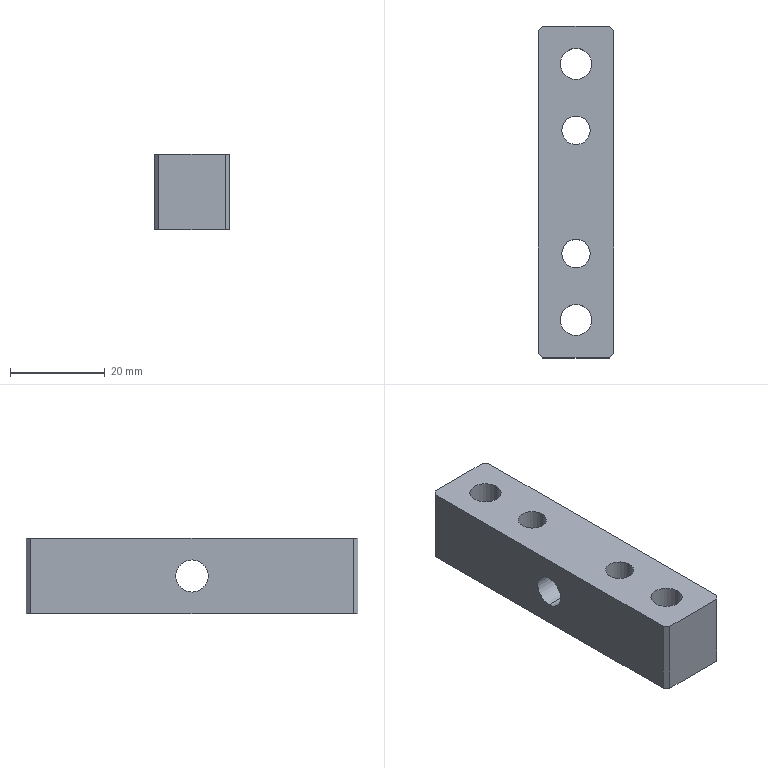Part | SolidWorks | features HoleWzd 3, Chamfer 1, ExtruThin 1 | 1 solid | 20 faces | box 16 x 70 x 16 mm | volume 15307 mm3 | cylinder 10 | plane 10 | commonest cylinder face diameters 6 x4 6.6 x4 6.8 x2
STEP:
#1=CARTESIAN_POINT('',(-11.3,62.,0.));
#2=VERTEX_POINT('',#1);
#3=CARTESIAN_POINT('',(-4.7,62.,0.));
#4=VERTEX_POINT('',#3);
#5=CARTESIAN_POINT('',(-8.,62.,0.));
#6=DIRECTION('',(0.,0.,1.));
#7=DIRECTION('',(1.,0.,0.));
#8=AXIS2_PLACEMENT_3D('',#5,#6,#7);
#9=CIRCLE('',#8,3.3);
#10=EDGE_CURVE('',#2,#4,#9,.T.);
#11=ORIENTED_EDGE('',*,*,#10,.F.);
#12=CARTESIAN_POINT('',(-11.3,62.,16.));
#13=VERTEX_POINT('',#12);
#14=CARTESIAN_POINT('',(-11.3,62.,16.));
#15=DIRECTION('',(0.,0.,1.));
#16=VECTOR('',#15,1000.);
#17=LINE('',#14,#16);
#18=EDGE_CURVE('',#2,#13,#17,.T.);
#19=ORIENTED_EDGE('',*,*,#18,.T.);
#20=CARTESIAN_POINT('',(-4.7,62.,16.));
#21=VERTEX_POINT('',#20);
#22=CARTESIAN_POINT('',(-8.,62.,16.));
#23=DIRECTION('',(0.,0.,1.));
#24=DIRECTION('',(1.,0.,0.));
#25=AXIS2_PLACEMENT_3D('',#22,#23,#24);
#26=CIRCLE('',#25,3.3);
#27=EDGE_CURVE('',#13,#21,#26,.T.);
#28=ORIENTED_EDGE('',*,*,#27,.T.);
#29=CARTESIAN_POINT('',(-4.7,62.,16.));
#30=DIRECTION('',(0.,0.,1.));
#31=VECTOR('',#30,1000.);
#32=LINE('',#29,#31);
#33=EDGE_CURVE('',#4,#21,#32,.T.);
#34=ORIENTED_EDGE('',*,*,#33,.F.);
#35=EDGE_LOOP('',(#11,#19,#28,#34));
#36=FACE_OUTER_BOUND('',#35,.T.);
#37=CARTESIAN_POINT('',(-8.,62.,16.));
#38=DIRECTION('',(0.,0.,1.));
#39=DIRECTION('',(1.,0.,0.));
#40=AXIS2_PLACEMENT_3D('',#37,#38,#39);
#41=CYLINDRICAL_SURFACE('',#40,3.3);
#42=ADVANCED_FACE('',(#36),#41,.F.);
#43=CARTESIAN_POINT('',(-11.3,8.,0.));
#44=VERTEX_POINT('',#43);
#45=CARTESIAN_POINT('',(-4.7,8.,0.));
#46=VERTEX_POINT('',#45);
#47=CARTESIAN_POINT('',(-8.,8.,0.));
#48=DIRECTION('',(0.,0.,1.));
#49=DIRECTION('',(1.,0.,0.));
#50=AXIS2_PLACEMENT_3D('',#47,#48,#49);
#51=CIRCLE('',#50,3.3);
#52=EDGE_CURVE('',#44,#46,#51,.T.);
#53=ORIENTED_EDGE('',*,*,#52,.F.);
#54=CARTESIAN_POINT('',(-11.3,8.,16.));
#55=VERTEX_POINT('',#54);
#56=CARTESIAN_POINT('',(-11.3,8.,16.));
#57=DIRECTION('',(0.,0.,1.));
#58=VECTOR('',#57,1000.);
#59=LINE('',#56,#58);
#60=EDGE_CURVE('',#44,#55,#59,.T.);
#61=ORIENTED_EDGE('',*,*,#60,.T.);
#62=CARTESIAN_POINT('',(-4.7,8.,16.));
#63=VERTEX_POINT('',#62);
#64=CARTESIAN_POINT('',(-8.,8.,16.));
#65=DIRECTION('',(0.,0.,1.));
#66=DIRECTION('',(1.,0.,0.));
#67=AXIS2_PLACEMENT_3D('',#64,#65,#66);
#68=CIRCLE('',#67,3.3);
#69=EDGE_CURVE('',#55,#63,#68,.T.);
#70=ORIENTED_EDGE('',*,*,#69,.T.);
#71=CARTESIAN_POINT('',(-4.7,8.,16.));
#72=DIRECTION('',(0.,0.,1.));
#73=VECTOR('',#72,1000.);
#74=LINE('',#71,#73);
#75=EDGE_CURVE('',#46,#63,#74,.T.);
#76=ORIENTED_EDGE('',*,*,#75,.F.);
#77=EDGE_LOOP('',(#53,#61,#70,#76));
#78=FACE_OUTER_BOUND('',#77,.T.);
#79=CARTESIAN_POINT('',(-8.,8.,16.));
#80=DIRECTION('',(0.,0.,1.));
#81=DIRECTION('',(1.,0.,0.));
#82=AXIS2_PLACEMENT_3D('',#79,#80,#81);
#83=CYLINDRICAL_SURFACE('',#82,3.3);
#84=ADVANCED_FACE('',(#78),#83,.F.);
#85=CARTESIAN_POINT('',(0.,35.,4.6));
#86=VERTEX_POINT('',#85);
#87=CARTESIAN_POINT('',(0.,35.,11.4));
#88=VERTEX_POINT('',#87);
#89=CARTESIAN_POINT('',(0.,35.,8.));
#90=DIRECTION('',(-1.,0.,0.));
#91=DIRECTION('',(0.,0.,1.));
#92=AXIS2_PLACEMENT_3D('',#89,#90,#91);
#93=CIRCLE('',#92,3.4);
#94=EDGE_CURVE('',#86,#88,#93,.T.);
#95=ORIENTED_EDGE('',*,*,#94,.F.);
#96=CARTESIAN_POINT('',(-16.,35.,4.6));
#97=VERTEX_POINT('',#96);
#98=CARTESIAN_POINT('',(-16.,35.,4.6));
#99=DIRECTION('',(-1.,0.,0.));
#100=VECTOR('',#99,1000.);
#101=LINE('',#98,#100);
#102=EDGE_CURVE('',#86,#97,#101,.T.);
#103=ORIENTED_EDGE('',*,*,#102,.T.);
#104=CARTESIAN_POINT('',(-16.,35.,11.4));
#105=VERTEX_POINT('',#104);
#106=CARTESIAN_POINT('',(-16.,35.,8.));
#107=DIRECTION('',(-1.,0.,0.));
#108=DIRECTION('',(0.,0.,1.));
#109=AXIS2_PLACEMENT_3D('',#106,#107,#108);
#110=CIRCLE('',#109,3.4);
#111=EDGE_CURVE('',#97,#105,#110,.T.);
#112=ORIENTED_EDGE('',*,*,#111,.T.);
#113=CARTESIAN_POINT('',(-16.,35.,11.4));
#114=DIRECTION('',(-1.,0.,0.));
#115=VECTOR('',#114,1000.);
#116=LINE('',#113,#115);
#117=EDGE_CURVE('',#88,#105,#116,.T.);
#118=ORIENTED_EDGE('',*,*,#117,.F.);
#119=EDGE_LOOP('',(#95,#103,#112,#118));
#120=FACE_OUTER_BOUND('',#119,.T.);
#121=CARTESIAN_POINT('',(-16.,35.,8.));
#122=DIRECTION('',(-1.,0.,0.));
#123=DIRECTION('',(0.,0.,1.));
#124=AXIS2_PLACEMENT_3D('',#121,#122,#123);
#125=CYLINDRICAL_SURFACE('',#124,3.4);
#126=ADVANCED_FACE('',(#120),#125,.F.);
#127=CARTESIAN_POINT('',(-11.,48.,0.));
#128=VERTEX_POINT('',#127);
#129=CARTESIAN_POINT('',(-5.,48.,0.));
#130=VERTEX_POINT('',#129);
#131=CARTESIAN_POINT('',(-8.,48.,0.));
#132=DIRECTION('',(0.,0.,1.));
#133=DIRECTION('',(1.,0.,0.));
#134=AXIS2_PLACEMENT_3D('',#131,#132,#133);
#135=CIRCLE('',#134,3.);
#136=EDGE_CURVE('',#128,#130,#135,.T.);
#137=ORIENTED_EDGE('',*,*,#136,.F.);
#138=CARTESIAN_POINT('',(-11.,48.,16.));
#139=VERTEX_POINT('',#138);
#140=CARTESIAN_POINT('',(-11.,48.,16.));
#141=DIRECTION('',(0.,0.,1.));
#142=VECTOR('',#141,1000.);
#143=LINE('',#140,#142);
#144=EDGE_CURVE('',#128,#139,#143,.T.);
#145=ORIENTED_EDGE('',*,*,#144,.T.);
#146=CARTESIAN_POINT('',(-5.,48.,16.));
#147=VERTEX_POINT('',#146);
#148=CARTESIAN_POINT('',(-8.,48.,16.));
#149=DIRECTION('',(0.,0.,1.));
#150=DIRECTION('',(1.,0.,0.));
#151=AXIS2_PLACEMENT_3D('',#148,#149,#150);
#152=CIRCLE('',#151,3.);
#153=EDGE_CURVE('',#139,#147,#152,.T.);
#154=ORIENTED_EDGE('',*,*,#153,.T.);
#155=CARTESIAN_POINT('',(-5.,48.,16.));
#156=DIRECTION('',(0.,0.,1.));
#157=VECTOR('',#156,1000.);
#158=LINE('',#155,#157);
#159=EDGE_CURVE('',#130,#147,#158,.T.);
#160=ORIENTED_EDGE('',*,*,#159,.F.);
#161=EDGE_LOOP('',(#137,#145,#154,#160));
#162=FACE_OUTER_BOUND('',#161,.T.);
#163=CARTESIAN_POINT('',(-8.,48.,16.));
#164=DIRECTION('',(0.,0.,1.));
#165=DIRECTION('',(1.,0.,0.));
#166=AXIS2_PLACEMENT_3D('',#163,#164,#165);
#167=CYLINDRICAL_SURFACE('',#166,3.);
#168=ADVANCED_FACE('',(#162),#167,.F.);
#169=CARTESIAN_POINT('',(-11.,22.,0.));
#170=VERTEX_POINT('',#169);
#171=CARTESIAN_POINT('',(-5.,22.,0.));
#172=VERTEX_POINT('',#171);
#173=CARTESIAN_POINT('',(-8.,22.,0.));
#174=DIRECTION('',(0.,0.,1.));
#175=DIRECTION('',(1.,0.,0.));
#176=AXIS2_PLACEMENT_3D('',#173,#174,#175);
#177=CIRCLE('',#176,3.);
#178=EDGE_CURVE('',#170,#172,#177,.T.);
#179=ORIENTED_EDGE('',*,*,#178,.F.);
#180=CARTESIAN_POINT('',(-11.,22.,16.));
#181=VERTEX_POINT('',#180);
#182=CARTESIAN_POINT('',(-11.,22.,16.));
#183=DIRECTION('',(0.,0.,1.));
#184=VECTOR('',#183,1000.);
#185=LINE('',#182,#184);
#186=EDGE_CURVE('',#170,#181,#185,.T.);
#187=ORIENTED_EDGE('',*,*,#186,.T.);
#188=CARTESIAN_POINT('',(-5.,22.,16.));
#189=VERTEX_POINT('',#188);
#190=CARTESIAN_POINT('',(-8.,22.,16.));
#191=DIRECTION('',(0.,0.,1.));
#192=DIRECTION('',(1.,0.,0.));
#193=AXIS2_PLACEMENT_3D('',#190,#191,#192);
#194=CIRCLE('',#193,3.);
#195=EDGE_CURVE('',#181,#189,#194,.T.);
#196=ORIENTED_EDGE('',*,*,#195,.T.);
#197=CARTESIAN_POINT('',(-5.,22.,16.));
#198=DIRECTION('',(0.,0.,1.));
#199=VECTOR('',#198,1000.);
#200=LINE('',#197,#199);
#201=EDGE_CURVE('',#172,#189,#200,.T.);
#202=ORIENTED_EDGE('',*,*,#201,.F.);
#203=EDGE_LOOP('',(#179,#187,#196,#202));
#204=FACE_OUTER_BOUND('',#203,.T.);
#205=CARTESIAN_POINT('',(-8.,22.,16.));
#206=DIRECTION('',(0.,0.,1.));
#207=DIRECTION('',(1.,0.,0.));
#208=AXIS2_PLACEMENT_3D('',#205,#206,#207);
#209=CYLINDRICAL_SURFACE('',#208,3.);
#210=ADVANCED_FACE('',(#204),#209,.F.);
#211=CARTESIAN_POINT('',(-16.,35.,8.));
#212=DIRECTION('',(-1.,0.,0.));
#213=DIRECTION('',(0.,0.,1.));
#214=AXIS2_PLACEMENT_3D('',#211,#212,#213);
#215=CIRCLE('',#214,3.4);
#216=EDGE_CURVE('',#105,#97,#215,.T.);
#217=ORIENTED_EDGE('',*,*,#216,.F.);
#218=ORIENTED_EDGE('',*,*,#111,.F.);
#219=EDGE_LOOP('',(#217,#218));
#220=FACE_BOUND('',#219,.T.);
#221=CARTESIAN_POINT('',(-16.,69.,16.));
#222=VERTEX_POINT('',#221);
#223=CARTESIAN_POINT('',(-16.,1.,16.));
#224=VERTEX_POINT('',#223);
#225=CARTESIAN_POINT('',(-16.,70.,16.));
#226=DIRECTION('',(0.,-1.,0.));
#227=VECTOR('',#226,1000.);
#228=LINE('',#225,#227);
#229=EDGE_CURVE('',#222,#224,#228,.T.);
#230=ORIENTED_EDGE('',*,*,#229,.F.);
#231=CARTESIAN_POINT('',(-16.,69.,0.));
#232=VERTEX_POINT('',#231);
#233=CARTESIAN_POINT('',(-16.,69.,0.));
#234=DIRECTION('',(0.,0.,-1.));
#235=VECTOR('',#234,1000.);
#236=LINE('',#233,#235);
#237=EDGE_CURVE('',#222,#232,#236,.T.);
#238=ORIENTED_EDGE('',*,*,#237,.T.);
#239=CARTESIAN_POINT('',(-16.,1.,0.));
#240=VERTEX_POINT('',#239);
#241=CARTESIAN_POINT('',(-16.,70.,0.));
#242=DIRECTION('',(0.,-1.,0.));
#243=VECTOR('',#242,1000.);
#244=LINE('',#241,#243);
#245=EDGE_CURVE('',#232,#240,#244,.T.);
#246=ORIENTED_EDGE('',*,*,#245,.T.);
#247=CARTESIAN_POINT('',(-16.,1.,16.));
#248=DIRECTION('',(0.,0.,1.));
#249=VECTOR('',#248,1000.);
#250=LINE('',#247,#249);
#251=EDGE_CURVE('',#240,#224,#250,.T.);
#252=ORIENTED_EDGE('',*,*,#251,.T.);
#253=EDGE_LOOP('',(#230,#238,#246,#252));
#254=FACE_OUTER_BOUND('',#253,.T.);
#255=CARTESIAN_POINT('',(-16.,70.,16.));
#256=DIRECTION('',(1.,0.,0.));
#257=DIRECTION('',(0.,1.,0.));
#258=AXIS2_PLACEMENT_3D('',#255,#256,#257);
#259=PLANE('',#258);
#260=ADVANCED_FACE('',(#220,#254),#259,.F.);
#261=CARTESIAN_POINT('',(-1.,0.,0.));
#262=VERTEX_POINT('',#261);
#263=CARTESIAN_POINT('',(-15.,0.,0.));
#264=VERTEX_POINT('',#263);
#265=CARTESIAN_POINT('',(0.,0.,0.));
#266=DIRECTION('',(-1.,0.,0.));
#267=VECTOR('',#266,1000.);
#268=LINE('',#265,#267);
#269=EDGE_CURVE('',#262,#264,#268,.T.);
#270=ORIENTED_EDGE('',*,*,#269,.F.);
#271=CARTESIAN_POINT('',(-1.,0.,16.));
#272=VERTEX_POINT('',#271);
#273=CARTESIAN_POINT('',(-1.,0.,16.));
#274=DIRECTION('',(0.,0.,1.));
#275=VECTOR('',#274,1000.);
#276=LINE('',#273,#275);
#277=EDGE_CURVE('',#262,#272,#276,.T.);
#278=ORIENTED_EDGE('',*,*,#277,.T.);
#279=CARTESIAN_POINT('',(-15.,0.,16.));
#280=VERTEX_POINT('',#279);
#281=CARTESIAN_POINT('',(0.,0.,16.));
#282=DIRECTION('',(-1.,0.,0.));
#283=VECTOR('',#282,1000.);
#284=LINE('',#281,#283);
#285=EDGE_CURVE('',#272,#280,#284,.T.);
#286=ORIENTED_EDGE('',*,*,#285,.T.);
#287=CARTESIAN_POINT('',(-15.,0.,0.));
#288=DIRECTION('',(0.,0.,-1.));
#289=VECTOR('',#288,1000.);
#290=LINE('',#287,#289);
#291=EDGE_CURVE('',#280,#264,#290,.T.);
#292=ORIENTED_EDGE('',*,*,#291,.T.);
#293=EDGE_LOOP('',(#270,#278,#286,#292));
#294=FACE_OUTER_BOUND('',#293,.T.);
#295=CARTESIAN_POINT('',(0.,0.,16.));
#296=DIRECTION('',(0.,-1.,0.));
#297=DIRECTION('',(0.,0.,-1.));
#298=AXIS2_PLACEMENT_3D('',#295,#296,#297);
#299=PLANE('',#298);
#300=ADVANCED_FACE('',(#294),#299,.T.);
#301=CARTESIAN_POINT('',(0.,35.,8.));
#302=DIRECTION('',(-1.,0.,0.));
#303=DIRECTION('',(0.,0.,1.));
#304=AXIS2_PLACEMENT_3D('',#301,#302,#303);
#305=CIRCLE('',#304,3.4);
#306=EDGE_CURVE('',#88,#86,#305,.T.);
#307=ORIENTED_EDGE('',*,*,#306,.T.);
#308=ORIENTED_EDGE('',*,*,#94,.T.);
#309=EDGE_LOOP('',(#307,#308));
#310=FACE_BOUND('',#309,.T.);
#311=CARTESIAN_POINT('',(0.,69.,0.));
#312=VERTEX_POINT('',#311);
#313=CARTESIAN_POINT('',(0.,1.,0.));
#314=VERTEX_POINT('',#313);
#315=CARTESIAN_POINT('',(0.,70.,0.));
#316=DIRECTION('',(0.,-1.,0.));
#317=VECTOR('',#316,1000.);
#318=LINE('',#315,#317);
#319=EDGE_CURVE('',#312,#314,#318,.T.);
#320=ORIENTED_EDGE('',*,*,#319,.F.);
#321=CARTESIAN_POINT('',(0.,69.,16.));
#322=VERTEX_POINT('',#321);
#323=CARTESIAN_POINT('',(0.,69.,16.));
#324=DIRECTION('',(0.,0.,1.));
#325=VECTOR('',#324,1000.);
#326=LINE('',#323,#325);
#327=EDGE_CURVE('',#312,#322,#326,.T.);
#328=ORIENTED_EDGE('',*,*,#327,.T.);
#329=CARTESIAN_POINT('',(0.,1.,16.));
#330=VERTEX_POINT('',#329);
#331=CARTESIAN_POINT('',(0.,70.,16.));
#332=DIRECTION('',(0.,-1.,0.));
#333=VECTOR('',#332,1000.);
#334=LINE('',#331,#333);
#335=EDGE_CURVE('',#322,#330,#334,.T.);
#336=ORIENTED_EDGE('',*,*,#335,.T.);
#337=CARTESIAN_POINT('',(0.,1.,16.));
#338=DIRECTION('',(0.,0.,-1.));
#339=VECTOR('',#338,1000.);
#340=LINE('',#337,#339);
#341=EDGE_CURVE('',#330,#314,#340,.T.);
#342=ORIENTED_EDGE('',*,*,#341,.T.);
#343=EDGE_LOOP('',(#320,#328,#336,#342));
#344=FACE_OUTER_BOUND('',#343,.T.);
#345=CARTESIAN_POINT('',(0.,70.,16.));
#346=DIRECTION('',(1.,0.,0.));
#347=DIRECTION('',(0.,1.,0.));
#348=AXIS2_PLACEMENT_3D('',#345,#346,#347);
#349=PLANE('',#348);
#350=ADVANCED_FACE('',(#310,#344),#349,.T.);
#351=CARTESIAN_POINT('',(-15.,70.,0.));
#352=VERTEX_POINT('',#351);
#353=CARTESIAN_POINT('',(-1.,70.,0.));
#354=VERTEX_POINT('',#353);
#355=CARTESIAN_POINT('',(-16.,70.,0.));
#356=DIRECTION('',(1.,0.,0.));
#357=VECTOR('',#356,1000.);
#358=LINE('',#355,#357);
#359=EDGE_CURVE('',#352,#354,#358,.T.);
#360=ORIENTED_EDGE('',*,*,#359,.F.);
#361=CARTESIAN_POINT('',(-15.,70.,16.));
#362=VERTEX_POINT('',#361);
#363=CARTESIAN_POINT('',(-15.,70.,16.));
#364=DIRECTION('',(0.,0.,1.));
#365=VECTOR('',#364,1000.);
#366=LINE('',#363,#365);
#367=EDGE_CURVE('',#352,#362,#366,.T.);
#368=ORIENTED_EDGE('',*,*,#367,.T.);
#369=CARTESIAN_POINT('',(-1.,70.,16.));
#370=VERTEX_POINT('',#369);
#371=CARTESIAN_POINT('',(-16.,70.,16.));
#372=DIRECTION('',(1.,0.,0.));
#373=VECTOR('',#372,1000.);
#374=LINE('',#371,#373);
#375=EDGE_CURVE('',#362,#370,#374,.T.);
#376=ORIENTED_EDGE('',*,*,#375,.T.);
#377=CARTESIAN_POINT('',(-1.,70.,16.));
#378=DIRECTION('',(0.,0.,-1.));
#379=VECTOR('',#378,1000.);
#380=LINE('',#377,#379);
#381=EDGE_CURVE('',#370,#354,#380,.T.);
#382=ORIENTED_EDGE('',*,*,#381,.T.);
#383=EDGE_LOOP('',(#360,#368,#376,#382));
#384=FACE_OUTER_BOUND('',#383,.T.);
#385=CARTESIAN_POINT('',(-16.,70.,16.));
#386=DIRECTION('',(0.,1.,0.));
#387=DIRECTION('',(0.,0.,1.));
#388=AXIS2_PLACEMENT_3D('',#385,#386,#387);
#389=PLANE('',#388);
#390=ADVANCED_FACE('',(#384),#389,.T.);
#391=CARTESIAN_POINT('',(-8.,62.,16.));
#392=DIRECTION('',(0.,0.,1.));
#393=DIRECTION('',(1.,0.,0.));
#394=AXIS2_PLACEMENT_3D('',#391,#392,#393);
#395=CIRCLE('',#394,3.3);
#396=EDGE_CURVE('',#21,#13,#395,.T.);
#397=ORIENTED_EDGE('',*,*,#396,.F.);
#398=ORIENTED_EDGE('',*,*,#27,.F.);
#399=EDGE_LOOP('',(#397,#398));
#400=FACE_BOUND('',#399,.T.);
#401=CARTESIAN_POINT('',(-8.,8.,16.));
#402=DIRECTION('',(0.,0.,1.));
#403=DIRECTION('',(1.,0.,0.));
#404=AXIS2_PLACEMENT_3D('',#401,#402,#403);
#405=CIRCLE('',#404,3.3);
#406=EDGE_CURVE('',#63,#55,#405,.T.);
#407=ORIENTED_EDGE('',*,*,#406,.F.);
#408=ORIENTED_EDGE('',*,*,#69,.F.);
#409=EDGE_LOOP('',(#407,#408));
#410=FACE_BOUND('',#409,.T.);
#411=CARTESIAN_POINT('',(-8.,48.,16.));
#412=DIRECTION('',(0.,0.,1.));
#413=DIRECTION('',(1.,0.,0.));
#414=AXIS2_PLACEMENT_3D('',#411,#412,#413);
#415=CIRCLE('',#414,3.);
#416=EDGE_CURVE('',#147,#139,#415,.T.);
#417=ORIENTED_EDGE('',*,*,#416,.F.);
#418=ORIENTED_EDGE('',*,*,#153,.F.);
#419=EDGE_LOOP('',(#417,#418));
#420=FACE_BOUND('',#419,.T.);
#421=CARTESIAN_POINT('',(-8.,22.,16.));
#422=DIRECTION('',(0.,0.,1.));
#423=DIRECTION('',(1.,0.,0.));
#424=AXIS2_PLACEMENT_3D('',#421,#422,#423);
#425=CIRCLE('',#424,3.);
#426=EDGE_CURVE('',#189,#181,#425,.T.);
#427=ORIENTED_EDGE('',*,*,#426,.F.);
#428=ORIENTED_EDGE('',*,*,#195,.F.);
#429=EDGE_LOOP('',(#427,#428));
#430=FACE_BOUND('',#429,.T.);
#431=ORIENTED_EDGE('',*,*,#375,.F.);
#432=CARTESIAN_POINT('',(-16.,69.,16.));
#433=DIRECTION('',(-0.7071,-0.7071,0.));
#434=VECTOR('',#433,1000.);
#435=LINE('',#432,#434);
#436=EDGE_CURVE('',#362,#222,#435,.T.);
#437=ORIENTED_EDGE('',*,*,#436,.T.);
#438=ORIENTED_EDGE('',*,*,#229,.T.);
#439=CARTESIAN_POINT('',(-15.,0.,16.));
#440=DIRECTION('',(0.7071,-0.7071,0.));
#441=VECTOR('',#440,1000.);
#442=LINE('',#439,#441);
#443=EDGE_CURVE('',#224,#280,#442,.T.);
#444=ORIENTED_EDGE('',*,*,#443,.T.);
#445=ORIENTED_EDGE('',*,*,#285,.F.);
#446=CARTESIAN_POINT('',(0.,1.,16.));
#447=DIRECTION('',(0.7071,0.7071,0.));
#448=VECTOR('',#447,1000.);
#449=LINE('',#446,#448);
#450=EDGE_CURVE('',#272,#330,#449,.T.);
#451=ORIENTED_EDGE('',*,*,#450,.T.);
#452=ORIENTED_EDGE('',*,*,#335,.F.);
#453=CARTESIAN_POINT('',(-1.,70.,16.));
#454=DIRECTION('',(-0.7071,0.7071,0.));
#455=VECTOR('',#454,1000.);
#456=LINE('',#453,#455);
#457=EDGE_CURVE('',#322,#370,#456,.T.);
#458=ORIENTED_EDGE('',*,*,#457,.T.);
#459=EDGE_LOOP('',(#431,#437,#438,#444,#445,#451,#452,#458));
#460=FACE_OUTER_BOUND('',#459,.T.);
#461=CARTESIAN_POINT('',(0.,0.,16.));
#462=DIRECTION('',(0.,0.,-1.));
#463=DIRECTION('',(-1.,0.,0.));
#464=AXIS2_PLACEMENT_3D('',#461,#462,#463);
#465=PLANE('',#464);
#466=ADVANCED_FACE('',(#400,#410,#420,#430,#460),#465,.F.);
#467=CARTESIAN_POINT('',(-8.,62.,0.));
#468=DIRECTION('',(0.,0.,1.));
#469=DIRECTION('',(1.,0.,0.));
#470=AXIS2_PLACEMENT_3D('',#467,#468,#469);
#471=CIRCLE('',#470,3.3);
#472=EDGE_CURVE('',#4,#2,#471,.T.);
#473=ORIENTED_EDGE('',*,*,#472,.T.);
#474=ORIENTED_EDGE('',*,*,#10,.T.);
#475=EDGE_LOOP('',(#473,#474));
#476=FACE_BOUND('',#475,.T.);
#477=CARTESIAN_POINT('',(-8.,8.,0.));
#478=DIRECTION('',(0.,0.,1.));
#479=DIRECTION('',(1.,0.,0.));
#480=AXIS2_PLACEMENT_3D('',#477,#478,#479);
#481=CIRCLE('',#480,3.3);
#482=EDGE_CURVE('',#46,#44,#481,.T.);
#483=ORIENTED_EDGE('',*,*,#482,.T.);
#484=ORIENTED_EDGE('',*,*,#52,.T.);
#485=EDGE_LOOP('',(#483,#484));
#486=FACE_BOUND('',#485,.T.);
#487=CARTESIAN_POINT('',(-8.,48.,0.));
#488=DIRECTION('',(0.,0.,1.));
#489=DIRECTION('',(1.,0.,0.));
#490=AXIS2_PLACEMENT_3D('',#487,#488,#489);
#491=CIRCLE('',#490,3.);
#492=EDGE_CURVE('',#130,#128,#491,.T.);
#493=ORIENTED_EDGE('',*,*,#492,.T.);
#494=ORIENTED_EDGE('',*,*,#136,.T.);
#495=EDGE_LOOP('',(#493,#494));
#496=FACE_BOUND('',#495,.T.);
#497=CARTESIAN_POINT('',(-8.,22.,0.));
#498=DIRECTION('',(0.,0.,1.));
#499=DIRECTION('',(1.,0.,0.));
#500=AXIS2_PLACEMENT_3D('',#497,#498,#499);
#501=CIRCLE('',#500,3.);
#502=EDGE_CURVE('',#172,#170,#501,.T.);
#503=ORIENTED_EDGE('',*,*,#502,.T.);
#504=ORIENTED_EDGE('',*,*,#178,.T.);
#505=EDGE_LOOP('',(#503,#504));
#506=FACE_BOUND('',#505,.T.);
#507=ORIENTED_EDGE('',*,*,#245,.F.);
#508=CARTESIAN_POINT('',(-42.5,42.5,0.));
#509=DIRECTION('',(0.7071,0.7071,0.));
#510=VECTOR('',#509,1000.);
#511=LINE('',#508,#510);
#512=EDGE_CURVE('',#232,#352,#511,.T.);
#513=ORIENTED_EDGE('',*,*,#512,.T.);
#514=ORIENTED_EDGE('',*,*,#359,.T.);
#515=CARTESIAN_POINT('',(34.5,34.5,0.));
#516=DIRECTION('',(0.7071,-0.7071,0.));
#517=VECTOR('',#516,1000.);
#518=LINE('',#515,#517);
#519=EDGE_CURVE('',#354,#312,#518,.T.);
#520=ORIENTED_EDGE('',*,*,#519,.T.);
#521=ORIENTED_EDGE('',*,*,#319,.T.);
#522=CARTESIAN_POINT('',(-0.5,0.5,0.));
#523=DIRECTION('',(-0.7071,-0.7071,0.));
#524=VECTOR('',#523,1000.);
#525=LINE('',#522,#524);
#526=EDGE_CURVE('',#314,#262,#525,.T.);
#527=ORIENTED_EDGE('',*,*,#526,.T.);
#528=ORIENTED_EDGE('',*,*,#269,.T.);
#529=CARTESIAN_POINT('',(-7.5,-7.5,0.));
#530=DIRECTION('',(-0.7071,0.7071,0.));
#531=VECTOR('',#530,1000.);
#532=LINE('',#529,#531);
#533=EDGE_CURVE('',#264,#240,#532,.T.);
#534=ORIENTED_EDGE('',*,*,#533,.T.);
#535=EDGE_LOOP('',(#507,#513,#514,#520,#521,#527,#528,#534));
#536=FACE_OUTER_BOUND('',#535,.T.);
#537=CARTESIAN_POINT('',(0.,0.,0.));
#538=DIRECTION('',(0.,0.,-1.));
#539=DIRECTION('',(-1.,0.,0.));
#540=AXIS2_PLACEMENT_3D('',#537,#538,#539);
#541=PLANE('',#540);
#542=ADVANCED_FACE('',(#476,#486,#496,#506,#536),#541,.T.);
#543=ORIENTED_EDGE('',*,*,#436,.F.);
#544=ORIENTED_EDGE('',*,*,#367,.F.);
#545=ORIENTED_EDGE('',*,*,#512,.F.);
#546=ORIENTED_EDGE('',*,*,#237,.F.);
#547=EDGE_LOOP('',(#543,#544,#545,#546));
#548=FACE_OUTER_BOUND('',#547,.T.);
#549=CARTESIAN_POINT('',(-16.,69.,16.));
#550=DIRECTION('',(-0.7071,0.7071,0.));
#551=DIRECTION('',(0.,0.,1.));
#552=AXIS2_PLACEMENT_3D('',#549,#550,#551);
#553=PLANE('',#552);
#554=ADVANCED_FACE('',(#548),#553,.T.);
#555=ORIENTED_EDGE('',*,*,#457,.F.);
#556=ORIENTED_EDGE('',*,*,#327,.F.);
#557=ORIENTED_EDGE('',*,*,#519,.F.);
#558=ORIENTED_EDGE('',*,*,#381,.F.);
#559=EDGE_LOOP('',(#555,#556,#557,#558));
#560=FACE_OUTER_BOUND('',#559,.T.);
#561=CARTESIAN_POINT('',(-1.,70.,16.));
#562=DIRECTION('',(-0.7071,-0.7071,0.));
#563=DIRECTION('',(0.,0.,-1.));
#564=AXIS2_PLACEMENT_3D('',#561,#562,#563);
#565=PLANE('',#564);
#566=ADVANCED_FACE('',(#560),#565,.F.);
#567=ORIENTED_EDGE('',*,*,#450,.F.);
#568=ORIENTED_EDGE('',*,*,#277,.F.);
#569=ORIENTED_EDGE('',*,*,#526,.F.);
#570=ORIENTED_EDGE('',*,*,#341,.F.);
#571=EDGE_LOOP('',(#567,#568,#569,#570));
#572=FACE_OUTER_BOUND('',#571,.T.);
#573=CARTESIAN_POINT('',(0.,1.,16.));
#574=DIRECTION('',(-0.7071,0.7071,0.));
#575=DIRECTION('',(0.,0.,-1.));
#576=AXIS2_PLACEMENT_3D('',#573,#574,#575);
#577=PLANE('',#576);
#578=ADVANCED_FACE('',(#572),#577,.F.);
#579=ORIENTED_EDGE('',*,*,#443,.F.);
#580=ORIENTED_EDGE('',*,*,#251,.F.);
#581=ORIENTED_EDGE('',*,*,#533,.F.);
#582=ORIENTED_EDGE('',*,*,#291,.F.);
#583=EDGE_LOOP('',(#579,#580,#581,#582));
#584=FACE_OUTER_BOUND('',#583,.T.);
#585=CARTESIAN_POINT('',(-15.,0.,16.));
#586=DIRECTION('',(-0.7071,-0.7071,0.));
#587=DIRECTION('',(0.,0.,1.));
#588=AXIS2_PLACEMENT_3D('',#585,#586,#587);
#589=PLANE('',#588);
#590=ADVANCED_FACE('',(#584),#589,.T.);
#591=ORIENTED_EDGE('',*,*,#186,.F.);
#592=ORIENTED_EDGE('',*,*,#502,.F.);
#593=ORIENTED_EDGE('',*,*,#201,.T.);
#594=ORIENTED_EDGE('',*,*,#426,.T.);
#595=EDGE_LOOP('',(#591,#592,#593,#594));
#596=FACE_OUTER_BOUND('',#595,.T.);
#597=CARTESIAN_POINT('',(-8.,22.,16.));
#598=DIRECTION('',(0.,0.,1.));
#599=DIRECTION('',(1.,0.,0.));
#600=AXIS2_PLACEMENT_3D('',#597,#598,#599);
#601=CYLINDRICAL_SURFACE('',#600,3.);
#602=ADVANCED_FACE('',(#596),#601,.F.);
#603=ORIENTED_EDGE('',*,*,#144,.F.);
#604=ORIENTED_EDGE('',*,*,#492,.F.);
#605=ORIENTED_EDGE('',*,*,#159,.T.);
#606=ORIENTED_EDGE('',*,*,#416,.T.);
#607=EDGE_LOOP('',(#603,#604,#605,#606));
#608=FACE_OUTER_BOUND('',#607,.T.);
#609=CARTESIAN_POINT('',(-8.,48.,16.));
#610=DIRECTION('',(0.,0.,1.));
#611=DIRECTION('',(1.,0.,0.));
#612=AXIS2_PLACEMENT_3D('',#609,#610,#611);
#613=CYLINDRICAL_SURFACE('',#612,3.);
#614=ADVANCED_FACE('',(#608),#613,.F.);
#615=ORIENTED_EDGE('',*,*,#102,.F.);
#616=ORIENTED_EDGE('',*,*,#306,.F.);
#617=ORIENTED_EDGE('',*,*,#117,.T.);
#618=ORIENTED_EDGE('',*,*,#216,.T.);
#619=EDGE_LOOP('',(#615,#616,#617,#618));
#620=FACE_OUTER_BOUND('',#619,.T.);
#621=CARTESIAN_POINT('',(-16.,35.,8.));
#622=DIRECTION('',(-1.,0.,0.));
#623=DIRECTION('',(0.,0.,1.));
#624=AXIS2_PLACEMENT_3D('',#621,#622,#623);
#625=CYLINDRICAL_SURFACE('',#624,3.4);
#626=ADVANCED_FACE('',(#620),#625,.F.);
#627=ORIENTED_EDGE('',*,*,#60,.F.);
#628=ORIENTED_EDGE('',*,*,#482,.F.);
#629=ORIENTED_EDGE('',*,*,#75,.T.);
#630=ORIENTED_EDGE('',*,*,#406,.T.);
#631=EDGE_LOOP('',(#627,#628,#629,#630));
#632=FACE_OUTER_BOUND('',#631,.T.);
#633=CARTESIAN_POINT('',(-8.,8.,16.));
#634=DIRECTION('',(0.,0.,1.));
#635=DIRECTION('',(1.,0.,0.));
#636=AXIS2_PLACEMENT_3D('',#633,#634,#635);
#637=CYLINDRICAL_SURFACE('',#636,3.3);
#638=ADVANCED_FACE('',(#632),#637,.F.);
#639=ORIENTED_EDGE('',*,*,#18,.F.);
#640=ORIENTED_EDGE('',*,*,#472,.F.);
#641=ORIENTED_EDGE('',*,*,#33,.T.);
#642=ORIENTED_EDGE('',*,*,#396,.T.);
#643=EDGE_LOOP('',(#639,#640,#641,#642));
#644=FACE_OUTER_BOUND('',#643,.T.);
#645=CARTESIAN_POINT('',(-8.,62.,16.));
#646=DIRECTION('',(0.,0.,1.));
#647=DIRECTION('',(1.,0.,0.));
#648=AXIS2_PLACEMENT_3D('',#645,#646,#647);
#649=CYLINDRICAL_SURFACE('',#648,3.3);
#650=ADVANCED_FACE('',(#644),#649,.F.);
#651=CLOSED_SHELL('',(#42,#84,#126,#168,#210,#260,#300,#350,#390,#466,#542,#554,#566,#578,#590,#602,#614,#626,#638,#650));
#652=MANIFOLD_SOLID_BREP('',#651);
#653=CARTESIAN_POINT('',(0.,0.,0.));
#654=DIRECTION('',(0.,0.,1.));
#655=DIRECTION('',(1.,0.,0.));
#656=AXIS2_PLACEMENT_3D('',#653,#654,#655);
#657=(LENGTH_UNIT()NAMED_UNIT(*)SI_UNIT(.MILLI.,.METRE.));
#658=UNCERTAINTY_MEASURE_WITH_UNIT(LENGTH_MEASURE(0.00001),#657,'','');
#659=(NAMED_UNIT(*)PLANE_ANGLE_UNIT()SI_UNIT($,.RADIAN.));
#660=(NAMED_UNIT(*)SI_UNIT($,.STERADIAN.)SOLID_ANGLE_UNIT());
#661=(GEOMETRIC_REPRESENTATION_CONTEXT(3)GLOBAL_UNCERTAINTY_ASSIGNED_CONTEXT((#658))GLOBAL_UNIT_ASSIGNED_CONTEXT((#657,#659,#660))REPRESENTATION_CONTEXT('',''));
#662=ADVANCED_BREP_SHAPE_REPRESENTATION('',(#652,#656),#661);